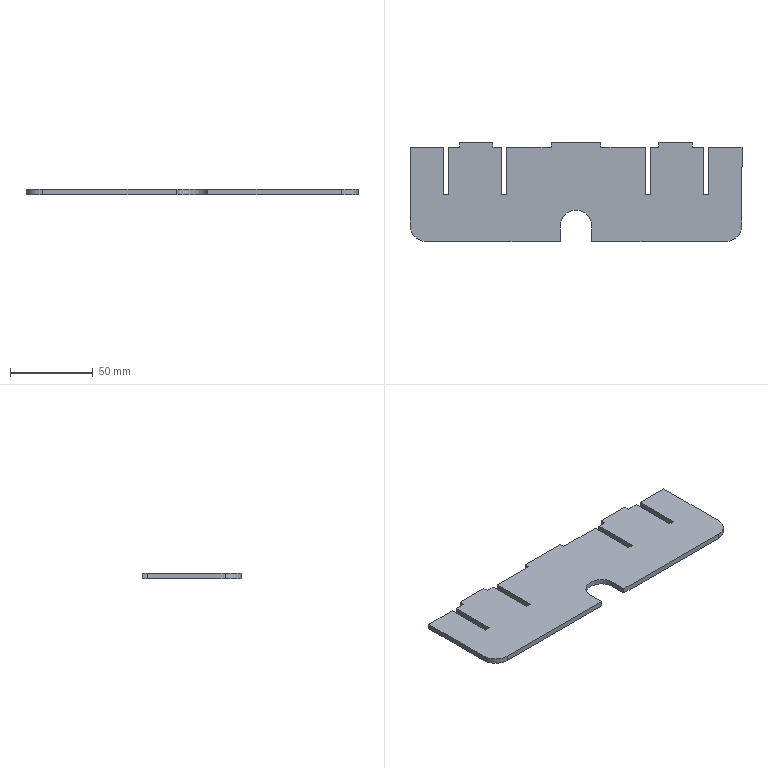Part | SolidWorks | features FlatPattern 1, SMBaseFlange 1, SheetMetal 1 | 1 solid | 40 faces | box 200 x 59.8 x 3.2 mm | volume 34688 mm3 | plane 37 | cylinder 3 | commonest cylinder face diameters 20 x2 19 x1
STEP:
#1=CARTESIAN_POINT('',(166.71,-150.,0.));
#2=VERTEX_POINT('',#1);
#3=CARTESIAN_POINT('',(166.71,-103.2,0.));
#4=VERTEX_POINT('',#3);
#5=CARTESIAN_POINT('',(166.71,-103.2,0.));
#6=DIRECTION('',(0.,1.,0.));
#7=VECTOR('',#6,1000.);
#8=LINE('',#5,#7);
#9=EDGE_CURVE('',#2,#4,#8,.T.);
#10=ORIENTED_EDGE('',*,*,#9,.F.);
#11=CARTESIAN_POINT('',(166.71,-150.,-3.2));
#12=VERTEX_POINT('',#11);
#13=CARTESIAN_POINT('',(166.71,-150.,-3.2));
#14=DIRECTION('',(0.,0.,1.));
#15=VECTOR('',#14,1000.);
#16=LINE('',#13,#15);
#17=EDGE_CURVE('',#12,#2,#16,.T.);
#18=ORIENTED_EDGE('',*,*,#17,.F.);
#19=CARTESIAN_POINT('',(166.71,-103.2,-3.2));
#20=VERTEX_POINT('',#19);
#21=CARTESIAN_POINT('',(166.71,-103.2,-3.2));
#22=DIRECTION('',(0.,1.,0.));
#23=VECTOR('',#22,1000.);
#24=LINE('',#21,#23);
#25=EDGE_CURVE('',#12,#20,#24,.T.);
#26=ORIENTED_EDGE('',*,*,#25,.T.);
#27=CARTESIAN_POINT('',(166.71,-103.2,-3.2));
#28=DIRECTION('',(0.,0.,1.));
#29=VECTOR('',#28,1000.);
#30=LINE('',#27,#29);
#31=EDGE_CURVE('',#20,#4,#30,.T.);
#32=ORIENTED_EDGE('',*,*,#31,.T.);
#33=EDGE_LOOP('',(#10,#18,#26,#32));
#34=FACE_OUTER_BOUND('',#33,.T.);
#35=CARTESIAN_POINT('',(166.71,-103.2,-3.2));
#36=DIRECTION('',(1.,0.,0.));
#37=DIRECTION('',(0.,1.,0.));
#38=AXIS2_PLACEMENT_3D('',#35,#36,#37);
#39=PLANE('',#38);
#40=ADVANCED_FACE('',(#34),#39,.T.);
#41=CARTESIAN_POINT('',(156.71,-160.,0.));
#42=VERTEX_POINT('',#41);
#43=CARTESIAN_POINT('',(156.71,-150.,0.));
#44=DIRECTION('',(0.,0.,1.));
#45=DIRECTION('',(-1.,0.,0.));
#46=AXIS2_PLACEMENT_3D('',#43,#44,#45);
#47=CIRCLE('',#46,10.);
#48=EDGE_CURVE('',#42,#2,#47,.T.);
#49=ORIENTED_EDGE('',*,*,#48,.F.);
#50=CARTESIAN_POINT('',(156.71,-160.,-3.2));
#51=VERTEX_POINT('',#50);
#52=CARTESIAN_POINT('',(156.71,-160.,-3.2));
#53=DIRECTION('',(0.,0.,1.));
#54=VECTOR('',#53,1000.);
#55=LINE('',#52,#54);
#56=EDGE_CURVE('',#51,#42,#55,.T.);
#57=ORIENTED_EDGE('',*,*,#56,.F.);
#58=CARTESIAN_POINT('',(156.71,-150.,-3.2));
#59=DIRECTION('',(0.,0.,1.));
#60=DIRECTION('',(-1.,0.,0.));
#61=AXIS2_PLACEMENT_3D('',#58,#59,#60);
#62=CIRCLE('',#61,10.);
#63=EDGE_CURVE('',#51,#12,#62,.T.);
#64=ORIENTED_EDGE('',*,*,#63,.T.);
#65=ORIENTED_EDGE('',*,*,#17,.T.);
#66=EDGE_LOOP('',(#49,#57,#64,#65));
#67=FACE_OUTER_BOUND('',#66,.T.);
#68=CARTESIAN_POINT('',(156.71,-150.,-3.2));
#69=DIRECTION('',(0.,0.,1.));
#70=DIRECTION('',(1.,0.,0.));
#71=AXIS2_PLACEMENT_3D('',#68,#69,#70);
#72=CYLINDRICAL_SURFACE('',#71,10.);
#73=ADVANCED_FACE('',(#67),#72,.T.);
#74=CARTESIAN_POINT('',(76.21,-160.,0.));
#75=VERTEX_POINT('',#74);
#76=CARTESIAN_POINT('',(156.71,-160.,0.));
#77=DIRECTION('',(1.,0.,0.));
#78=VECTOR('',#77,1000.);
#79=LINE('',#76,#78);
#80=EDGE_CURVE('',#75,#42,#79,.T.);
#81=ORIENTED_EDGE('',*,*,#80,.F.);
#82=CARTESIAN_POINT('',(76.21,-160.,-3.2));
#83=VERTEX_POINT('',#82);
#84=CARTESIAN_POINT('',(76.21,-160.,-3.2));
#85=DIRECTION('',(0.,0.,1.));
#86=VECTOR('',#85,1000.);
#87=LINE('',#84,#86);
#88=EDGE_CURVE('',#83,#75,#87,.T.);
#89=ORIENTED_EDGE('',*,*,#88,.F.);
#90=CARTESIAN_POINT('',(156.71,-160.,-3.2));
#91=DIRECTION('',(1.,0.,0.));
#92=VECTOR('',#91,1000.);
#93=LINE('',#90,#92);
#94=EDGE_CURVE('',#83,#51,#93,.T.);
#95=ORIENTED_EDGE('',*,*,#94,.T.);
#96=ORIENTED_EDGE('',*,*,#56,.T.);
#97=EDGE_LOOP('',(#81,#89,#95,#96));
#98=FACE_OUTER_BOUND('',#97,.T.);
#99=CARTESIAN_POINT('',(156.71,-160.,-3.2));
#100=DIRECTION('',(0.,-1.,0.));
#101=DIRECTION('',(0.,0.,-1.));
#102=AXIS2_PLACEMENT_3D('',#99,#100,#101);
#103=PLANE('',#102);
#104=ADVANCED_FACE('',(#98),#103,.T.);
#105=CARTESIAN_POINT('',(76.21,-150.5,0.));
#106=VERTEX_POINT('',#105);
#107=CARTESIAN_POINT('',(76.21,-160.,0.));
#108=DIRECTION('',(0.,-1.,0.));
#109=VECTOR('',#108,1000.);
#110=LINE('',#107,#109);
#111=EDGE_CURVE('',#106,#75,#110,.T.);
#112=ORIENTED_EDGE('',*,*,#111,.F.);
#113=CARTESIAN_POINT('',(76.21,-150.5,-3.2));
#114=VERTEX_POINT('',#113);
#115=CARTESIAN_POINT('',(76.21,-150.5,-3.2));
#116=DIRECTION('',(0.,0.,1.));
#117=VECTOR('',#116,1000.);
#118=LINE('',#115,#117);
#119=EDGE_CURVE('',#114,#106,#118,.T.);
#120=ORIENTED_EDGE('',*,*,#119,.F.);
#121=CARTESIAN_POINT('',(76.21,-160.,-3.2));
#122=DIRECTION('',(0.,-1.,0.));
#123=VECTOR('',#122,1000.);
#124=LINE('',#121,#123);
#125=EDGE_CURVE('',#114,#83,#124,.T.);
#126=ORIENTED_EDGE('',*,*,#125,.T.);
#127=ORIENTED_EDGE('',*,*,#88,.T.);
#128=EDGE_LOOP('',(#112,#120,#126,#127));
#129=FACE_OUTER_BOUND('',#128,.T.);
#130=CARTESIAN_POINT('',(76.21,-160.,-3.2));
#131=DIRECTION('',(-1.,0.,0.));
#132=DIRECTION('',(0.,-1.,0.));
#133=AXIS2_PLACEMENT_3D('',#130,#131,#132);
#134=PLANE('',#133);
#135=ADVANCED_FACE('',(#129),#134,.T.);
#136=CARTESIAN_POINT('',(57.21,-150.5,0.));
#137=VERTEX_POINT('',#136);
#138=CARTESIAN_POINT('',(66.71,-150.5,0.));
#139=DIRECTION('',(0.,0.,-1.));
#140=DIRECTION('',(1.,0.,0.));
#141=AXIS2_PLACEMENT_3D('',#138,#139,#140);
#142=CIRCLE('',#141,9.5);
#143=EDGE_CURVE('',#137,#106,#142,.T.);
#144=ORIENTED_EDGE('',*,*,#143,.F.);
#145=CARTESIAN_POINT('',(57.21,-150.5,-3.2));
#146=VERTEX_POINT('',#145);
#147=CARTESIAN_POINT('',(57.21,-150.5,-3.2));
#148=DIRECTION('',(0.,0.,1.));
#149=VECTOR('',#148,1000.);
#150=LINE('',#147,#149);
#151=EDGE_CURVE('',#146,#137,#150,.T.);
#152=ORIENTED_EDGE('',*,*,#151,.F.);
#153=CARTESIAN_POINT('',(66.71,-150.5,-3.2));
#154=DIRECTION('',(0.,0.,-1.));
#155=DIRECTION('',(1.,0.,0.));
#156=AXIS2_PLACEMENT_3D('',#153,#154,#155);
#157=CIRCLE('',#156,9.5);
#158=EDGE_CURVE('',#146,#114,#157,.T.);
#159=ORIENTED_EDGE('',*,*,#158,.T.);
#160=ORIENTED_EDGE('',*,*,#119,.T.);
#161=EDGE_LOOP('',(#144,#152,#159,#160));
#162=FACE_OUTER_BOUND('',#161,.T.);
#163=CARTESIAN_POINT('',(66.71,-150.5,-3.2));
#164=DIRECTION('',(0.,0.,1.));
#165=DIRECTION('',(1.,0.,0.));
#166=AXIS2_PLACEMENT_3D('',#163,#164,#165);
#167=CYLINDRICAL_SURFACE('',#166,9.5);
#168=ADVANCED_FACE('',(#162),#167,.F.);
#169=CARTESIAN_POINT('',(57.21,-160.,0.));
#170=VERTEX_POINT('',#169);
#171=CARTESIAN_POINT('',(57.21,-150.5,0.));
#172=DIRECTION('',(0.,1.,0.));
#173=VECTOR('',#172,1000.);
#174=LINE('',#171,#173);
#175=EDGE_CURVE('',#170,#137,#174,.T.);
#176=ORIENTED_EDGE('',*,*,#175,.F.);
#177=CARTESIAN_POINT('',(57.21,-160.,-3.2));
#178=VERTEX_POINT('',#177);
#179=CARTESIAN_POINT('',(57.21,-160.,-3.2));
#180=DIRECTION('',(0.,0.,1.));
#181=VECTOR('',#180,1000.);
#182=LINE('',#179,#181);
#183=EDGE_CURVE('',#178,#170,#182,.T.);
#184=ORIENTED_EDGE('',*,*,#183,.F.);
#185=CARTESIAN_POINT('',(57.21,-150.5,-3.2));
#186=DIRECTION('',(0.,1.,0.));
#187=VECTOR('',#186,1000.);
#188=LINE('',#185,#187);
#189=EDGE_CURVE('',#178,#146,#188,.T.);
#190=ORIENTED_EDGE('',*,*,#189,.T.);
#191=ORIENTED_EDGE('',*,*,#151,.T.);
#192=EDGE_LOOP('',(#176,#184,#190,#191));
#193=FACE_OUTER_BOUND('',#192,.T.);
#194=CARTESIAN_POINT('',(57.21,-150.5,-3.2));
#195=DIRECTION('',(1.,0.,0.));
#196=DIRECTION('',(0.,1.,0.));
#197=AXIS2_PLACEMENT_3D('',#194,#195,#196);
#198=PLANE('',#197);
#199=ADVANCED_FACE('',(#193),#198,.T.);
#200=CARTESIAN_POINT('',(-23.29,-160.,0.));
#201=VERTEX_POINT('',#200);
#202=CARTESIAN_POINT('',(57.21,-160.,0.));
#203=DIRECTION('',(1.,0.,0.));
#204=VECTOR('',#203,1000.);
#205=LINE('',#202,#204);
#206=EDGE_CURVE('',#201,#170,#205,.T.);
#207=ORIENTED_EDGE('',*,*,#206,.F.);
#208=CARTESIAN_POINT('',(-23.29,-160.,-3.2));
#209=VERTEX_POINT('',#208);
#210=CARTESIAN_POINT('',(-23.29,-160.,-3.2));
#211=DIRECTION('',(0.,0.,1.));
#212=VECTOR('',#211,1000.);
#213=LINE('',#210,#212);
#214=EDGE_CURVE('',#209,#201,#213,.T.);
#215=ORIENTED_EDGE('',*,*,#214,.F.);
#216=CARTESIAN_POINT('',(57.21,-160.,-3.2));
#217=DIRECTION('',(1.,0.,0.));
#218=VECTOR('',#217,1000.);
#219=LINE('',#216,#218);
#220=EDGE_CURVE('',#209,#178,#219,.T.);
#221=ORIENTED_EDGE('',*,*,#220,.T.);
#222=ORIENTED_EDGE('',*,*,#183,.T.);
#223=EDGE_LOOP('',(#207,#215,#221,#222));
#224=FACE_OUTER_BOUND('',#223,.T.);
#225=CARTESIAN_POINT('',(57.21,-160.,-3.2));
#226=DIRECTION('',(0.,-1.,0.));
#227=DIRECTION('',(0.,0.,-1.));
#228=AXIS2_PLACEMENT_3D('',#225,#226,#227);
#229=PLANE('',#228);
#230=ADVANCED_FACE('',(#224),#229,.T.);
#231=CARTESIAN_POINT('',(-33.29,-150.,0.));
#232=VERTEX_POINT('',#231);
#233=CARTESIAN_POINT('',(-23.29,-150.,0.));
#234=DIRECTION('',(0.,0.,1.));
#235=DIRECTION('',(-1.,0.,0.));
#236=AXIS2_PLACEMENT_3D('',#233,#234,#235);
#237=CIRCLE('',#236,10.);
#238=EDGE_CURVE('',#232,#201,#237,.T.);
#239=ORIENTED_EDGE('',*,*,#238,.F.);
#240=CARTESIAN_POINT('',(-33.29,-150.,-3.2));
#241=VERTEX_POINT('',#240);
#242=CARTESIAN_POINT('',(-33.29,-150.,-3.2));
#243=DIRECTION('',(0.,0.,1.));
#244=VECTOR('',#243,1000.);
#245=LINE('',#242,#244);
#246=EDGE_CURVE('',#241,#232,#245,.T.);
#247=ORIENTED_EDGE('',*,*,#246,.F.);
#248=CARTESIAN_POINT('',(-23.29,-150.,-3.2));
#249=DIRECTION('',(0.,0.,1.));
#250=DIRECTION('',(-1.,0.,0.));
#251=AXIS2_PLACEMENT_3D('',#248,#249,#250);
#252=CIRCLE('',#251,10.);
#253=EDGE_CURVE('',#241,#209,#252,.T.);
#254=ORIENTED_EDGE('',*,*,#253,.T.);
#255=ORIENTED_EDGE('',*,*,#214,.T.);
#256=EDGE_LOOP('',(#239,#247,#254,#255));
#257=FACE_OUTER_BOUND('',#256,.T.);
#258=CARTESIAN_POINT('',(-23.29,-150.,-3.2));
#259=DIRECTION('',(0.,0.,1.));
#260=DIRECTION('',(1.,0.,0.));
#261=AXIS2_PLACEMENT_3D('',#258,#259,#260);
#262=CYLINDRICAL_SURFACE('',#261,10.);
#263=ADVANCED_FACE('',(#257),#262,.T.);
#264=CARTESIAN_POINT('',(-33.29,-103.2,0.));
#265=VERTEX_POINT('',#264);
#266=CARTESIAN_POINT('',(-33.29,-103.2,0.));
#267=DIRECTION('',(0.,-1.,0.));
#268=VECTOR('',#267,1000.);
#269=LINE('',#266,#268);
#270=EDGE_CURVE('',#265,#232,#269,.T.);
#271=ORIENTED_EDGE('',*,*,#270,.F.);
#272=CARTESIAN_POINT('',(-33.29,-103.2,-3.2));
#273=VERTEX_POINT('',#272);
#274=CARTESIAN_POINT('',(-33.29,-103.2,-3.2));
#275=DIRECTION('',(0.,0.,1.));
#276=VECTOR('',#275,1000.);
#277=LINE('',#274,#276);
#278=EDGE_CURVE('',#273,#265,#277,.T.);
#279=ORIENTED_EDGE('',*,*,#278,.F.);
#280=CARTESIAN_POINT('',(-33.29,-103.2,-3.2));
#281=DIRECTION('',(0.,-1.,0.));
#282=VECTOR('',#281,1000.);
#283=LINE('',#280,#282);
#284=EDGE_CURVE('',#273,#241,#283,.T.);
#285=ORIENTED_EDGE('',*,*,#284,.T.);
#286=ORIENTED_EDGE('',*,*,#246,.T.);
#287=EDGE_LOOP('',(#271,#279,#285,#286));
#288=FACE_OUTER_BOUND('',#287,.T.);
#289=CARTESIAN_POINT('',(-33.29,-103.2,-3.2));
#290=DIRECTION('',(-1.,0.,0.));
#291=DIRECTION('',(0.,-1.,0.));
#292=AXIS2_PLACEMENT_3D('',#289,#290,#291);
#293=PLANE('',#292);
#294=ADVANCED_FACE('',(#288),#293,.T.);
#295=CARTESIAN_POINT('',(-13.29,-103.2,0.));
#296=VERTEX_POINT('',#295);
#297=CARTESIAN_POINT('',(-13.29,-103.2,0.));
#298=DIRECTION('',(-1.,0.,0.));
#299=VECTOR('',#298,1000.);
#300=LINE('',#297,#299);
#301=EDGE_CURVE('',#296,#265,#300,.T.);
#302=ORIENTED_EDGE('',*,*,#301,.F.);
#303=CARTESIAN_POINT('',(-13.29,-103.2,-3.2));
#304=VERTEX_POINT('',#303);
#305=CARTESIAN_POINT('',(-13.29,-103.2,-3.2));
#306=DIRECTION('',(0.,0.,1.));
#307=VECTOR('',#306,1000.);
#308=LINE('',#305,#307);
#309=EDGE_CURVE('',#304,#296,#308,.T.);
#310=ORIENTED_EDGE('',*,*,#309,.F.);
#311=CARTESIAN_POINT('',(-13.29,-103.2,-3.2));
#312=DIRECTION('',(-1.,0.,0.));
#313=VECTOR('',#312,1000.);
#314=LINE('',#311,#313);
#315=EDGE_CURVE('',#304,#273,#314,.T.);
#316=ORIENTED_EDGE('',*,*,#315,.T.);
#317=ORIENTED_EDGE('',*,*,#278,.T.);
#318=EDGE_LOOP('',(#302,#310,#316,#317));
#319=FACE_OUTER_BOUND('',#318,.T.);
#320=CARTESIAN_POINT('',(-13.29,-103.2,-3.2));
#321=DIRECTION('',(0.,1.,0.));
#322=DIRECTION('',(-1.,0.,0.));
#323=AXIS2_PLACEMENT_3D('',#320,#321,#322);
#324=PLANE('',#323);
#325=ADVANCED_FACE('',(#319),#324,.T.);
#326=CARTESIAN_POINT('',(-13.29,-131.7,0.));
#327=VERTEX_POINT('',#326);
#328=CARTESIAN_POINT('',(-13.29,-131.7,0.));
#329=DIRECTION('',(0.,1.,0.));
#330=VECTOR('',#329,1000.);
#331=LINE('',#328,#330);
#332=EDGE_CURVE('',#327,#296,#331,.T.);
#333=ORIENTED_EDGE('',*,*,#332,.F.);
#334=CARTESIAN_POINT('',(-13.29,-131.7,-3.2));
#335=VERTEX_POINT('',#334);
#336=CARTESIAN_POINT('',(-13.29,-131.7,-3.2));
#337=DIRECTION('',(0.,0.,1.));
#338=VECTOR('',#337,1000.);
#339=LINE('',#336,#338);
#340=EDGE_CURVE('',#335,#327,#339,.T.);
#341=ORIENTED_EDGE('',*,*,#340,.F.);
#342=CARTESIAN_POINT('',(-13.29,-131.7,-3.2));
#343=DIRECTION('',(0.,1.,0.));
#344=VECTOR('',#343,1000.);
#345=LINE('',#342,#344);
#346=EDGE_CURVE('',#335,#304,#345,.T.);
#347=ORIENTED_EDGE('',*,*,#346,.T.);
#348=ORIENTED_EDGE('',*,*,#309,.T.);
#349=EDGE_LOOP('',(#333,#341,#347,#348));
#350=FACE_OUTER_BOUND('',#349,.T.);
#351=CARTESIAN_POINT('',(-13.29,-131.7,-3.2));
#352=DIRECTION('',(1.,0.,0.));
#353=DIRECTION('',(0.,1.,0.));
#354=AXIS2_PLACEMENT_3D('',#351,#352,#353);
#355=PLANE('',#354);
#356=ADVANCED_FACE('',(#350),#355,.T.);
#357=CARTESIAN_POINT('',(-10.09,-131.7,0.));
#358=VERTEX_POINT('',#357);
#359=CARTESIAN_POINT('',(-10.09,-131.7,0.));
#360=DIRECTION('',(-1.,0.,0.));
#361=VECTOR('',#360,1000.);
#362=LINE('',#359,#361);
#363=EDGE_CURVE('',#358,#327,#362,.T.);
#364=ORIENTED_EDGE('',*,*,#363,.F.);
#365=CARTESIAN_POINT('',(-10.09,-131.7,-3.2));
#366=VERTEX_POINT('',#365);
#367=CARTESIAN_POINT('',(-10.09,-131.7,-3.2));
#368=DIRECTION('',(0.,0.,1.));
#369=VECTOR('',#368,1000.);
#370=LINE('',#367,#369);
#371=EDGE_CURVE('',#366,#358,#370,.T.);
#372=ORIENTED_EDGE('',*,*,#371,.F.);
#373=CARTESIAN_POINT('',(-10.09,-131.7,-3.2));
#374=DIRECTION('',(-1.,0.,0.));
#375=VECTOR('',#374,1000.);
#376=LINE('',#373,#375);
#377=EDGE_CURVE('',#366,#335,#376,.T.);
#378=ORIENTED_EDGE('',*,*,#377,.T.);
#379=ORIENTED_EDGE('',*,*,#340,.T.);
#380=EDGE_LOOP('',(#364,#372,#378,#379));
#381=FACE_OUTER_BOUND('',#380,.T.);
#382=CARTESIAN_POINT('',(-10.09,-131.7,-3.2));
#383=DIRECTION('',(0.,1.,0.));
#384=DIRECTION('',(0.,0.,1.));
#385=AXIS2_PLACEMENT_3D('',#382,#383,#384);
#386=PLANE('',#385);
#387=ADVANCED_FACE('',(#381),#386,.T.);
#388=CARTESIAN_POINT('',(-10.09,-103.2,0.));
#389=VERTEX_POINT('',#388);
#390=CARTESIAN_POINT('',(-10.09,-103.2,0.));
#391=DIRECTION('',(0.,-1.,0.));
#392=VECTOR('',#391,1000.);
#393=LINE('',#390,#392);
#394=EDGE_CURVE('',#389,#358,#393,.T.);
#395=ORIENTED_EDGE('',*,*,#394,.F.);
#396=CARTESIAN_POINT('',(-10.09,-103.2,-3.2));
#397=VERTEX_POINT('',#396);
#398=CARTESIAN_POINT('',(-10.09,-103.2,-3.2));
#399=DIRECTION('',(0.,0.,1.));
#400=VECTOR('',#399,1000.);
#401=LINE('',#398,#400);
#402=EDGE_CURVE('',#397,#389,#401,.T.);
#403=ORIENTED_EDGE('',*,*,#402,.F.);
#404=CARTESIAN_POINT('',(-10.09,-103.2,-3.2));
#405=DIRECTION('',(0.,-1.,0.));
#406=VECTOR('',#405,1000.);
#407=LINE('',#404,#406);
#408=EDGE_CURVE('',#397,#366,#407,.T.);
#409=ORIENTED_EDGE('',*,*,#408,.T.);
#410=ORIENTED_EDGE('',*,*,#371,.T.);
#411=EDGE_LOOP('',(#395,#403,#409,#410));
#412=FACE_OUTER_BOUND('',#411,.T.);
#413=CARTESIAN_POINT('',(-10.09,-103.2,-3.2));
#414=DIRECTION('',(-1.,0.,0.));
#415=DIRECTION('',(0.,-1.,0.));
#416=AXIS2_PLACEMENT_3D('',#413,#414,#415);
#417=PLANE('',#416);
#418=ADVANCED_FACE('',(#412),#417,.T.);
#419=CARTESIAN_POINT('',(-3.29,-103.2,0.));
#420=VERTEX_POINT('',#419);
#421=CARTESIAN_POINT('',(-3.29,-103.2,0.));
#422=DIRECTION('',(-1.,0.,0.));
#423=VECTOR('',#422,1000.);
#424=LINE('',#421,#423);
#425=EDGE_CURVE('',#420,#389,#424,.T.);
#426=ORIENTED_EDGE('',*,*,#425,.F.);
#427=CARTESIAN_POINT('',(-3.29,-103.2,-3.2));
#428=VERTEX_POINT('',#427);
#429=CARTESIAN_POINT('',(-3.29,-103.2,-3.2));
#430=DIRECTION('',(0.,0.,1.));
#431=VECTOR('',#430,1000.);
#432=LINE('',#429,#431);
#433=EDGE_CURVE('',#428,#420,#432,.T.);
#434=ORIENTED_EDGE('',*,*,#433,.F.);
#435=CARTESIAN_POINT('',(-3.29,-103.2,-3.2));
#436=DIRECTION('',(-1.,0.,0.));
#437=VECTOR('',#436,1000.);
#438=LINE('',#435,#437);
#439=EDGE_CURVE('',#428,#397,#438,.T.);
#440=ORIENTED_EDGE('',*,*,#439,.T.);
#441=ORIENTED_EDGE('',*,*,#402,.T.);
#442=EDGE_LOOP('',(#426,#434,#440,#441));
#443=FACE_OUTER_BOUND('',#442,.T.);
#444=CARTESIAN_POINT('',(-3.29,-103.2,-3.2));
#445=DIRECTION('',(0.,1.,0.));
#446=DIRECTION('',(-1.,0.,0.));
#447=AXIS2_PLACEMENT_3D('',#444,#445,#446);
#448=PLANE('',#447);
#449=ADVANCED_FACE('',(#443),#448,.T.);
#450=CARTESIAN_POINT('',(-3.29,-100.2,0.));
#451=VERTEX_POINT('',#450);
#452=CARTESIAN_POINT('',(-3.29,-100.2,0.));
#453=DIRECTION('',(0.,-1.,0.));
#454=VECTOR('',#453,1000.);
#455=LINE('',#452,#454);
#456=EDGE_CURVE('',#451,#420,#455,.T.);
#457=ORIENTED_EDGE('',*,*,#456,.F.);
#458=CARTESIAN_POINT('',(-3.29,-100.2,-3.2));
#459=VERTEX_POINT('',#458);
#460=CARTESIAN_POINT('',(-3.29,-100.2,-3.2));
#461=DIRECTION('',(0.,0.,1.));
#462=VECTOR('',#461,1000.);
#463=LINE('',#460,#462);
#464=EDGE_CURVE('',#459,#451,#463,.T.);
#465=ORIENTED_EDGE('',*,*,#464,.F.);
#466=CARTESIAN_POINT('',(-3.29,-100.2,-3.2));
#467=DIRECTION('',(0.,-1.,0.));
#468=VECTOR('',#467,1000.);
#469=LINE('',#466,#468);
#470=EDGE_CURVE('',#459,#428,#469,.T.);
#471=ORIENTED_EDGE('',*,*,#470,.T.);
#472=ORIENTED_EDGE('',*,*,#433,.T.);
#473=EDGE_LOOP('',(#457,#465,#471,#472));
#474=FACE_OUTER_BOUND('',#473,.T.);
#475=CARTESIAN_POINT('',(-3.29,-100.2,-3.2));
#476=DIRECTION('',(-1.,0.,0.));
#477=DIRECTION('',(0.,-1.,0.));
#478=AXIS2_PLACEMENT_3D('',#475,#476,#477);
#479=PLANE('',#478);
#480=ADVANCED_FACE('',(#474),#479,.T.);
#481=CARTESIAN_POINT('',(16.71,-100.2,0.));
#482=VERTEX_POINT('',#481);
#483=CARTESIAN_POINT('',(16.71,-100.2,0.));
#484=DIRECTION('',(-1.,0.,0.));
#485=VECTOR('',#484,1000.);
#486=LINE('',#483,#485);
#487=EDGE_CURVE('',#482,#451,#486,.T.);
#488=ORIENTED_EDGE('',*,*,#487,.F.);
#489=CARTESIAN_POINT('',(16.71,-100.2,-3.2));
#490=VERTEX_POINT('',#489);
#491=CARTESIAN_POINT('',(16.71,-100.2,-3.2));
#492=DIRECTION('',(0.,0.,1.));
#493=VECTOR('',#492,1000.);
#494=LINE('',#491,#493);
#495=EDGE_CURVE('',#490,#482,#494,.T.);
#496=ORIENTED_EDGE('',*,*,#495,.F.);
#497=CARTESIAN_POINT('',(16.71,-100.2,-3.2));
#498=DIRECTION('',(-1.,0.,0.));
#499=VECTOR('',#498,1000.);
#500=LINE('',#497,#499);
#501=EDGE_CURVE('',#490,#459,#500,.T.);
#502=ORIENTED_EDGE('',*,*,#501,.T.);
#503=ORIENTED_EDGE('',*,*,#464,.T.);
#504=EDGE_LOOP('',(#488,#496,#502,#503));
#505=FACE_OUTER_BOUND('',#504,.T.);
#506=CARTESIAN_POINT('',(16.71,-100.2,-3.2));
#507=DIRECTION('',(0.,1.,0.));
#508=DIRECTION('',(0.,0.,1.));
#509=AXIS2_PLACEMENT_3D('',#506,#507,#508);
#510=PLANE('',#509);
#511=ADVANCED_FACE('',(#505),#510,.T.);
#512=CARTESIAN_POINT('',(16.71,-103.2,0.));
#513=VERTEX_POINT('',#512);
#514=CARTESIAN_POINT('',(16.71,-103.2,0.));
#515=DIRECTION('',(0.,1.,0.));
#516=VECTOR('',#515,1000.);
#517=LINE('',#514,#516);
#518=EDGE_CURVE('',#513,#482,#517,.T.);
#519=ORIENTED_EDGE('',*,*,#518,.F.);
#520=CARTESIAN_POINT('',(16.71,-103.2,-3.2));
#521=VERTEX_POINT('',#520);
#522=CARTESIAN_POINT('',(16.71,-103.2,-3.2));
#523=DIRECTION('',(0.,0.,1.));
#524=VECTOR('',#523,1000.);
#525=LINE('',#522,#524);
#526=EDGE_CURVE('',#521,#513,#525,.T.);
#527=ORIENTED_EDGE('',*,*,#526,.F.);
#528=CARTESIAN_POINT('',(16.71,-103.2,-3.2));
#529=DIRECTION('',(0.,1.,0.));
#530=VECTOR('',#529,1000.);
#531=LINE('',#528,#530);
#532=EDGE_CURVE('',#521,#490,#531,.T.);
#533=ORIENTED_EDGE('',*,*,#532,.T.);
#534=ORIENTED_EDGE('',*,*,#495,.T.);
#535=EDGE_LOOP('',(#519,#527,#533,#534));
#536=FACE_OUTER_BOUND('',#535,.T.);
#537=CARTESIAN_POINT('',(16.71,-103.2,-3.2));
#538=DIRECTION('',(1.,0.,0.));
#539=DIRECTION('',(0.,0.,-1.));
#540=AXIS2_PLACEMENT_3D('',#537,#538,#539);
#541=PLANE('',#540);
#542=ADVANCED_FACE('',(#536),#541,.T.);
#543=CARTESIAN_POINT('',(21.71,-103.2,0.));
#544=VERTEX_POINT('',#543);
#545=CARTESIAN_POINT('',(21.71,-103.2,0.));
#546=DIRECTION('',(-1.,0.,0.));
#547=VECTOR('',#546,1000.);
#548=LINE('',#545,#547);
#549=EDGE_CURVE('',#544,#513,#548,.T.);
#550=ORIENTED_EDGE('',*,*,#549,.F.);
#551=CARTESIAN_POINT('',(21.71,-103.2,-3.2));
#552=VERTEX_POINT('',#551);
#553=CARTESIAN_POINT('',(21.71,-103.2,-3.2));
#554=DIRECTION('',(0.,0.,1.));
#555=VECTOR('',#554,1000.);
#556=LINE('',#553,#555);
#557=EDGE_CURVE('',#552,#544,#556,.T.);
#558=ORIENTED_EDGE('',*,*,#557,.F.);
#559=CARTESIAN_POINT('',(21.71,-103.2,-3.2));
#560=DIRECTION('',(-1.,0.,0.));
#561=VECTOR('',#560,1000.);
#562=LINE('',#559,#561);
#563=EDGE_CURVE('',#552,#521,#562,.T.);
#564=ORIENTED_EDGE('',*,*,#563,.T.);
#565=ORIENTED_EDGE('',*,*,#526,.T.);
#566=EDGE_LOOP('',(#550,#558,#564,#565));
#567=FACE_OUTER_BOUND('',#566,.T.);
#568=CARTESIAN_POINT('',(21.71,-103.2,-3.2));
#569=DIRECTION('',(0.,1.,0.));
#570=DIRECTION('',(-1.,0.,0.));
#571=AXIS2_PLACEMENT_3D('',#568,#569,#570);
#572=PLANE('',#571);
#573=ADVANCED_FACE('',(#567),#572,.T.);
#574=CARTESIAN_POINT('',(21.71,-131.7,0.));
#575=VERTEX_POINT('',#574);
#576=CARTESIAN_POINT('',(21.71,-131.7,0.));
#577=DIRECTION('',(0.,1.,0.));
#578=VECTOR('',#577,1000.);
#579=LINE('',#576,#578);
#580=EDGE_CURVE('',#575,#544,#579,.T.);
#581=ORIENTED_EDGE('',*,*,#580,.F.);
#582=CARTESIAN_POINT('',(21.71,-131.7,-3.2));
#583=VERTEX_POINT('',#582);
#584=CARTESIAN_POINT('',(21.71,-131.7,-3.2));
#585=DIRECTION('',(0.,0.,1.));
#586=VECTOR('',#585,1000.);
#587=LINE('',#584,#586);
#588=EDGE_CURVE('',#583,#575,#587,.T.);
#589=ORIENTED_EDGE('',*,*,#588,.F.);
#590=CARTESIAN_POINT('',(21.71,-131.7,-3.2));
#591=DIRECTION('',(0.,1.,0.));
#592=VECTOR('',#591,1000.);
#593=LINE('',#590,#592);
#594=EDGE_CURVE('',#583,#552,#593,.T.);
#595=ORIENTED_EDGE('',*,*,#594,.T.);
#596=ORIENTED_EDGE('',*,*,#557,.T.);
#597=EDGE_LOOP('',(#581,#589,#595,#596));
#598=FACE_OUTER_BOUND('',#597,.T.);
#599=CARTESIAN_POINT('',(21.71,-131.7,-3.2));
#600=DIRECTION('',(1.,0.,0.));
#601=DIRECTION('',(0.,1.,0.));
#602=AXIS2_PLACEMENT_3D('',#599,#600,#601);
#603=PLANE('',#602);
#604=ADVANCED_FACE('',(#598),#603,.T.);
#605=CARTESIAN_POINT('',(24.91,-131.7,0.));
#606=VERTEX_POINT('',#605);
#607=CARTESIAN_POINT('',(24.91,-131.7,0.));
#608=DIRECTION('',(-1.,0.,0.));
#609=VECTOR('',#608,1000.);
#610=LINE('',#607,#609);
#611=EDGE_CURVE('',#606,#575,#610,.T.);
#612=ORIENTED_EDGE('',*,*,#611,.F.);
#613=CARTESIAN_POINT('',(24.91,-131.7,-3.2));
#614=VERTEX_POINT('',#613);
#615=CARTESIAN_POINT('',(24.91,-131.7,-3.2));
#616=DIRECTION('',(0.,0.,1.));
#617=VECTOR('',#616,1000.);
#618=LINE('',#615,#617);
#619=EDGE_CURVE('',#614,#606,#618,.T.);
#620=ORIENTED_EDGE('',*,*,#619,.F.);
#621=CARTESIAN_POINT('',(24.91,-131.7,-3.2));
#622=DIRECTION('',(-1.,0.,0.));
#623=VECTOR('',#622,1000.);
#624=LINE('',#621,#623);
#625=EDGE_CURVE('',#614,#583,#624,.T.);
#626=ORIENTED_EDGE('',*,*,#625,.T.);
#627=ORIENTED_EDGE('',*,*,#588,.T.);
#628=EDGE_LOOP('',(#612,#620,#626,#627));
#629=FACE_OUTER_BOUND('',#628,.T.);
#630=CARTESIAN_POINT('',(24.91,-131.7,-3.2));
#631=DIRECTION('',(0.,1.,0.));
#632=DIRECTION('',(0.,0.,1.));
#633=AXIS2_PLACEMENT_3D('',#630,#631,#632);
#634=PLANE('',#633);
#635=ADVANCED_FACE('',(#629),#634,.T.);
#636=CARTESIAN_POINT('',(24.91,-103.2,0.));
#637=VERTEX_POINT('',#636);
#638=CARTESIAN_POINT('',(24.91,-103.2,0.));
#639=DIRECTION('',(0.,-1.,0.));
#640=VECTOR('',#639,1000.);
#641=LINE('',#638,#640);
#642=EDGE_CURVE('',#637,#606,#641,.T.);
#643=ORIENTED_EDGE('',*,*,#642,.F.);
#644=CARTESIAN_POINT('',(24.91,-103.2,-3.2));
#645=VERTEX_POINT('',#644);
#646=CARTESIAN_POINT('',(24.91,-103.2,-3.2));
#647=DIRECTION('',(0.,0.,1.));
#648=VECTOR('',#647,1000.);
#649=LINE('',#646,#648);
#650=EDGE_CURVE('',#645,#637,#649,.T.);
#651=ORIENTED_EDGE('',*,*,#650,.F.);
#652=CARTESIAN_POINT('',(24.91,-103.2,-3.2));
#653=DIRECTION('',(0.,-1.,0.));
#654=VECTOR('',#653,1000.);
#655=LINE('',#652,#654);
#656=EDGE_CURVE('',#645,#614,#655,.T.);
#657=ORIENTED_EDGE('',*,*,#656,.T.);
#658=ORIENTED_EDGE('',*,*,#619,.T.);
#659=EDGE_LOOP('',(#643,#651,#657,#658));
#660=FACE_OUTER_BOUND('',#659,.T.);
#661=CARTESIAN_POINT('',(24.91,-103.2,-3.2));
#662=DIRECTION('',(-1.,0.,0.));
#663=DIRECTION('',(0.,-1.,0.));
#664=AXIS2_PLACEMENT_3D('',#661,#662,#663);
#665=PLANE('',#664);
#666=ADVANCED_FACE('',(#660),#665,.T.);
#667=CARTESIAN_POINT('',(51.71,-103.2,0.));
#668=VERTEX_POINT('',#667);
#669=CARTESIAN_POINT('',(51.71,-103.2,0.));
#670=DIRECTION('',(-1.,0.,0.));
#671=VECTOR('',#670,1000.);
#672=LINE('',#669,#671);
#673=EDGE_CURVE('',#668,#637,#672,.T.);
#674=ORIENTED_EDGE('',*,*,#673,.F.);
#675=CARTESIAN_POINT('',(51.71,-103.2,-3.2));
#676=VERTEX_POINT('',#675);
#677=CARTESIAN_POINT('',(51.71,-103.2,-3.2));
#678=DIRECTION('',(0.,0.,1.));
#679=VECTOR('',#678,1000.);
#680=LINE('',#677,#679);
#681=EDGE_CURVE('',#676,#668,#680,.T.);
#682=ORIENTED_EDGE('',*,*,#681,.F.);
#683=CARTESIAN_POINT('',(51.71,-103.2,-3.2));
#684=DIRECTION('',(-1.,0.,0.));
#685=VECTOR('',#684,1000.);
#686=LINE('',#683,#685);
#687=EDGE_CURVE('',#676,#645,#686,.T.);
#688=ORIENTED_EDGE('',*,*,#687,.T.);
#689=ORIENTED_EDGE('',*,*,#650,.T.);
#690=EDGE_LOOP('',(#674,#682,#688,#689));
#691=FACE_OUTER_BOUND('',#690,.T.);
#692=CARTESIAN_POINT('',(51.71,-103.2,-3.2));
#693=DIRECTION('',(0.,1.,0.));
#694=DIRECTION('',(-1.,0.,0.));
#695=AXIS2_PLACEMENT_3D('',#692,#693,#694);
#696=PLANE('',#695);
#697=ADVANCED_FACE('',(#691),#696,.T.);
#698=CARTESIAN_POINT('',(51.71,-100.2,0.));
#699=VERTEX_POINT('',#698);
#700=CARTESIAN_POINT('',(51.71,-100.2,0.));
#701=DIRECTION('',(0.,-1.,0.));
#702=VECTOR('',#701,1000.);
#703=LINE('',#700,#702);
#704=EDGE_CURVE('',#699,#668,#703,.T.);
#705=ORIENTED_EDGE('',*,*,#704,.F.);
#706=CARTESIAN_POINT('',(51.71,-100.2,-3.2));
#707=VERTEX_POINT('',#706);
#708=CARTESIAN_POINT('',(51.71,-100.2,-3.2));
#709=DIRECTION('',(0.,0.,1.));
#710=VECTOR('',#709,1000.);
#711=LINE('',#708,#710);
#712=EDGE_CURVE('',#707,#699,#711,.T.);
#713=ORIENTED_EDGE('',*,*,#712,.F.);
#714=CARTESIAN_POINT('',(51.71,-100.2,-3.2));
#715=DIRECTION('',(0.,-1.,0.));
#716=VECTOR('',#715,1000.);
#717=LINE('',#714,#716);
#718=EDGE_CURVE('',#707,#676,#717,.T.);
#719=ORIENTED_EDGE('',*,*,#718,.T.);
#720=ORIENTED_EDGE('',*,*,#681,.T.);
#721=EDGE_LOOP('',(#705,#713,#719,#720));
#722=FACE_OUTER_BOUND('',#721,.T.);
#723=CARTESIAN_POINT('',(51.71,-100.2,-3.2));
#724=DIRECTION('',(-1.,0.,0.));
#725=DIRECTION('',(0.,0.,1.));
#726=AXIS2_PLACEMENT_3D('',#723,#724,#725);
#727=PLANE('',#726);
#728=ADVANCED_FACE('',(#722),#727,.T.);
#729=CARTESIAN_POINT('',(81.71,-100.2,0.));
#730=VERTEX_POINT('',#729);
#731=CARTESIAN_POINT('',(81.71,-100.2,0.));
#732=DIRECTION('',(-1.,0.,0.));
#733=VECTOR('',#732,1000.);
#734=LINE('',#731,#733);
#735=EDGE_CURVE('',#730,#699,#734,.T.);
#736=ORIENTED_EDGE('',*,*,#735,.F.);
#737=CARTESIAN_POINT('',(81.71,-100.2,-3.2));
#738=VERTEX_POINT('',#737);
#739=CARTESIAN_POINT('',(81.71,-100.2,-3.2));
#740=DIRECTION('',(0.,0.,1.));
#741=VECTOR('',#740,1000.);
#742=LINE('',#739,#741);
#743=EDGE_CURVE('',#738,#730,#742,.T.);
#744=ORIENTED_EDGE('',*,*,#743,.F.);
#745=CARTESIAN_POINT('',(81.71,-100.2,-3.2));
#746=DIRECTION('',(-1.,0.,0.));
#747=VECTOR('',#746,1000.);
#748=LINE('',#745,#747);
#749=EDGE_CURVE('',#738,#707,#748,.T.);
#750=ORIENTED_EDGE('',*,*,#749,.T.);
#751=ORIENTED_EDGE('',*,*,#712,.T.);
#752=EDGE_LOOP('',(#736,#744,#750,#751));
#753=FACE_OUTER_BOUND('',#752,.T.);
#754=CARTESIAN_POINT('',(81.71,-100.2,-3.2));
#755=DIRECTION('',(0.,1.,0.));
#756=DIRECTION('',(0.,0.,1.));
#757=AXIS2_PLACEMENT_3D('',#754,#755,#756);
#758=PLANE('',#757);
#759=ADVANCED_FACE('',(#753),#758,.T.);
#760=CARTESIAN_POINT('',(81.71,-103.2,0.));
#761=VERTEX_POINT('',#760);
#762=CARTESIAN_POINT('',(81.71,-103.2,0.));
#763=DIRECTION('',(0.,1.,0.));
#764=VECTOR('',#763,1000.);
#765=LINE('',#762,#764);
#766=EDGE_CURVE('',#761,#730,#765,.T.);
#767=ORIENTED_EDGE('',*,*,#766,.F.);
#768=CARTESIAN_POINT('',(81.71,-103.2,-3.2));
#769=VERTEX_POINT('',#768);
#770=CARTESIAN_POINT('',(81.71,-103.2,-3.2));
#771=DIRECTION('',(0.,0.,1.));
#772=VECTOR('',#771,1000.);
#773=LINE('',#770,#772);
#774=EDGE_CURVE('',#769,#761,#773,.T.);
#775=ORIENTED_EDGE('',*,*,#774,.F.);
#776=CARTESIAN_POINT('',(81.71,-103.2,-3.2));
#777=DIRECTION('',(0.,1.,0.));
#778=VECTOR('',#777,1000.);
#779=LINE('',#776,#778);
#780=EDGE_CURVE('',#769,#738,#779,.T.);
#781=ORIENTED_EDGE('',*,*,#780,.T.);
#782=ORIENTED_EDGE('',*,*,#743,.T.);
#783=EDGE_LOOP('',(#767,#775,#781,#782));
#784=FACE_OUTER_BOUND('',#783,.T.);
#785=CARTESIAN_POINT('',(81.71,-103.2,-3.2));
#786=DIRECTION('',(1.,0.,0.));
#787=DIRECTION('',(0.,0.,-1.));
#788=AXIS2_PLACEMENT_3D('',#785,#786,#787);
#789=PLANE('',#788);
#790=ADVANCED_FACE('',(#784),#789,.T.);
#791=CARTESIAN_POINT('',(108.51,-103.2,0.));
#792=VERTEX_POINT('',#791);
#793=CARTESIAN_POINT('',(108.51,-103.2,0.));
#794=DIRECTION('',(-1.,0.,0.));
#795=VECTOR('',#794,1000.);
#796=LINE('',#793,#795);
#797=EDGE_CURVE('',#792,#761,#796,.T.);
#798=ORIENTED_EDGE('',*,*,#797,.F.);
#799=CARTESIAN_POINT('',(108.51,-103.2,-3.2));
#800=VERTEX_POINT('',#799);
#801=CARTESIAN_POINT('',(108.51,-103.2,-3.2));
#802=DIRECTION('',(0.,0.,1.));
#803=VECTOR('',#802,1000.);
#804=LINE('',#801,#803);
#805=EDGE_CURVE('',#800,#792,#804,.T.);
#806=ORIENTED_EDGE('',*,*,#805,.F.);
#807=CARTESIAN_POINT('',(108.51,-103.2,-3.2));
#808=DIRECTION('',(-1.,0.,0.));
#809=VECTOR('',#808,1000.);
#810=LINE('',#807,#809);
#811=EDGE_CURVE('',#800,#769,#810,.T.);
#812=ORIENTED_EDGE('',*,*,#811,.T.);
#813=ORIENTED_EDGE('',*,*,#774,.T.);
#814=EDGE_LOOP('',(#798,#806,#812,#813));
#815=FACE_OUTER_BOUND('',#814,.T.);
#816=CARTESIAN_POINT('',(108.51,-103.2,-3.2));
#817=DIRECTION('',(0.,1.,0.));
#818=DIRECTION('',(-1.,0.,0.));
#819=AXIS2_PLACEMENT_3D('',#816,#817,#818);
#820=PLANE('',#819);
#821=ADVANCED_FACE('',(#815),#820,.T.);
#822=CARTESIAN_POINT('',(108.51,-131.7,0.));
#823=VERTEX_POINT('',#822);
#824=CARTESIAN_POINT('',(108.51,-131.7,0.));
#825=DIRECTION('',(0.,1.,0.));
#826=VECTOR('',#825,1000.);
#827=LINE('',#824,#826);
#828=EDGE_CURVE('',#823,#792,#827,.T.);
#829=ORIENTED_EDGE('',*,*,#828,.F.);
#830=CARTESIAN_POINT('',(108.51,-131.7,-3.2));
#831=VERTEX_POINT('',#830);
#832=CARTESIAN_POINT('',(108.51,-131.7,-3.2));
#833=DIRECTION('',(0.,0.,1.));
#834=VECTOR('',#833,1000.);
#835=LINE('',#832,#834);
#836=EDGE_CURVE('',#831,#823,#835,.T.);
#837=ORIENTED_EDGE('',*,*,#836,.F.);
#838=CARTESIAN_POINT('',(108.51,-131.7,-3.2));
#839=DIRECTION('',(0.,1.,0.));
#840=VECTOR('',#839,1000.);
#841=LINE('',#838,#840);
#842=EDGE_CURVE('',#831,#800,#841,.T.);
#843=ORIENTED_EDGE('',*,*,#842,.T.);
#844=ORIENTED_EDGE('',*,*,#805,.T.);
#845=EDGE_LOOP('',(#829,#837,#843,#844));
#846=FACE_OUTER_BOUND('',#845,.T.);
#847=CARTESIAN_POINT('',(108.51,-131.7,-3.2));
#848=DIRECTION('',(1.,0.,0.));
#849=DIRECTION('',(0.,1.,0.));
#850=AXIS2_PLACEMENT_3D('',#847,#848,#849);
#851=PLANE('',#850);
#852=ADVANCED_FACE('',(#846),#851,.T.);
#853=CARTESIAN_POINT('',(111.71,-131.7,0.));
#854=VERTEX_POINT('',#853);
#855=CARTESIAN_POINT('',(111.71,-131.7,0.));
#856=DIRECTION('',(-1.,0.,0.));
#857=VECTOR('',#856,1000.);
#858=LINE('',#855,#857);
#859=EDGE_CURVE('',#854,#823,#858,.T.);
#860=ORIENTED_EDGE('',*,*,#859,.F.);
#861=CARTESIAN_POINT('',(111.71,-131.7,-3.2));
#862=VERTEX_POINT('',#861);
#863=CARTESIAN_POINT('',(111.71,-131.7,-3.2));
#864=DIRECTION('',(0.,0.,1.));
#865=VECTOR('',#864,1000.);
#866=LINE('',#863,#865);
#867=EDGE_CURVE('',#862,#854,#866,.T.);
#868=ORIENTED_EDGE('',*,*,#867,.F.);
#869=CARTESIAN_POINT('',(111.71,-131.7,-3.2));
#870=DIRECTION('',(-1.,0.,0.));
#871=VECTOR('',#870,1000.);
#872=LINE('',#869,#871);
#873=EDGE_CURVE('',#862,#831,#872,.T.);
#874=ORIENTED_EDGE('',*,*,#873,.T.);
#875=ORIENTED_EDGE('',*,*,#836,.T.);
#876=EDGE_LOOP('',(#860,#868,#874,#875));
#877=FACE_OUTER_BOUND('',#876,.T.);
#878=CARTESIAN_POINT('',(111.71,-131.7,-3.2));
#879=DIRECTION('',(0.,1.,0.));
#880=DIRECTION('',(0.,0.,1.));
#881=AXIS2_PLACEMENT_3D('',#878,#879,#880);
#882=PLANE('',#881);
#883=ADVANCED_FACE('',(#877),#882,.T.);
#884=CARTESIAN_POINT('',(111.71,-103.2,0.));
#885=VERTEX_POINT('',#884);
#886=CARTESIAN_POINT('',(111.71,-103.2,0.));
#887=DIRECTION('',(0.,-1.,0.));
#888=VECTOR('',#887,1000.);
#889=LINE('',#886,#888);
#890=EDGE_CURVE('',#885,#854,#889,.T.);
#891=ORIENTED_EDGE('',*,*,#890,.F.);
#892=CARTESIAN_POINT('',(111.71,-103.2,-3.2));
#893=VERTEX_POINT('',#892);
#894=CARTESIAN_POINT('',(111.71,-103.2,-3.2));
#895=DIRECTION('',(0.,0.,1.));
#896=VECTOR('',#895,1000.);
#897=LINE('',#894,#896);
#898=EDGE_CURVE('',#893,#885,#897,.T.);
#899=ORIENTED_EDGE('',*,*,#898,.F.);
#900=CARTESIAN_POINT('',(111.71,-103.2,-3.2));
#901=DIRECTION('',(0.,-1.,0.));
#902=VECTOR('',#901,1000.);
#903=LINE('',#900,#902);
#904=EDGE_CURVE('',#893,#862,#903,.T.);
#905=ORIENTED_EDGE('',*,*,#904,.T.);
#906=ORIENTED_EDGE('',*,*,#867,.T.);
#907=EDGE_LOOP('',(#891,#899,#905,#906));
#908=FACE_OUTER_BOUND('',#907,.T.);
#909=CARTESIAN_POINT('',(111.71,-103.2,-3.2));
#910=DIRECTION('',(-1.,0.,0.));
#911=DIRECTION('',(0.,-1.,0.));
#912=AXIS2_PLACEMENT_3D('',#909,#910,#911);
#913=PLANE('',#912);
#914=ADVANCED_FACE('',(#908),#913,.T.);
#915=CARTESIAN_POINT('',(116.71,-103.2,0.));
#916=VERTEX_POINT('',#915);
#917=CARTESIAN_POINT('',(116.71,-103.2,0.));
#918=DIRECTION('',(-1.,0.,0.));
#919=VECTOR('',#918,1000.);
#920=LINE('',#917,#919);
#921=EDGE_CURVE('',#916,#885,#920,.T.);
#922=ORIENTED_EDGE('',*,*,#921,.F.);
#923=CARTESIAN_POINT('',(116.71,-103.2,-3.2));
#924=VERTEX_POINT('',#923);
#925=CARTESIAN_POINT('',(116.71,-103.2,-3.2));
#926=DIRECTION('',(0.,0.,1.));
#927=VECTOR('',#926,1000.);
#928=LINE('',#925,#927);
#929=EDGE_CURVE('',#924,#916,#928,.T.);
#930=ORIENTED_EDGE('',*,*,#929,.F.);
#931=CARTESIAN_POINT('',(116.71,-103.2,-3.2));
#932=DIRECTION('',(-1.,0.,0.));
#933=VECTOR('',#932,1000.);
#934=LINE('',#931,#933);
#935=EDGE_CURVE('',#924,#893,#934,.T.);
#936=ORIENTED_EDGE('',*,*,#935,.T.);
#937=ORIENTED_EDGE('',*,*,#898,.T.);
#938=EDGE_LOOP('',(#922,#930,#936,#937));
#939=FACE_OUTER_BOUND('',#938,.T.);
#940=CARTESIAN_POINT('',(116.71,-103.2,-3.2));
#941=DIRECTION('',(0.,1.,0.));
#942=DIRECTION('',(-1.,0.,0.));
#943=AXIS2_PLACEMENT_3D('',#940,#941,#942);
#944=PLANE('',#943);
#945=ADVANCED_FACE('',(#939),#944,.T.);
#946=CARTESIAN_POINT('',(116.71,-100.2,0.));
#947=VERTEX_POINT('',#946);
#948=CARTESIAN_POINT('',(116.71,-100.2,0.));
#949=DIRECTION('',(0.,-1.,0.));
#950=VECTOR('',#949,1000.);
#951=LINE('',#948,#950);
#952=EDGE_CURVE('',#947,#916,#951,.T.);
#953=ORIENTED_EDGE('',*,*,#952,.F.);
#954=CARTESIAN_POINT('',(116.71,-100.2,-3.2));
#955=VERTEX_POINT('',#954);
#956=CARTESIAN_POINT('',(116.71,-100.2,-3.2));
#957=DIRECTION('',(0.,0.,1.));
#958=VECTOR('',#957,1000.);
#959=LINE('',#956,#958);
#960=EDGE_CURVE('',#955,#947,#959,.T.);
#961=ORIENTED_EDGE('',*,*,#960,.F.);
#962=CARTESIAN_POINT('',(116.71,-100.2,-3.2));
#963=DIRECTION('',(0.,-1.,0.));
#964=VECTOR('',#963,1000.);
#965=LINE('',#962,#964);
#966=EDGE_CURVE('',#955,#924,#965,.T.);
#967=ORIENTED_EDGE('',*,*,#966,.T.);
#968=ORIENTED_EDGE('',*,*,#929,.T.);
#969=EDGE_LOOP('',(#953,#961,#967,#968));
#970=FACE_OUTER_BOUND('',#969,.T.);
#971=CARTESIAN_POINT('',(116.71,-100.2,-3.2));
#972=DIRECTION('',(-1.,0.,0.));
#973=DIRECTION('',(0.,0.,1.));
#974=AXIS2_PLACEMENT_3D('',#971,#972,#973);
#975=PLANE('',#974);
#976=ADVANCED_FACE('',(#970),#975,.T.);
#977=CARTESIAN_POINT('',(136.71,-100.2,0.));
#978=VERTEX_POINT('',#977);
#979=CARTESIAN_POINT('',(136.71,-100.2,0.));
#980=DIRECTION('',(-1.,0.,0.));
#981=VECTOR('',#980,1000.);
#982=LINE('',#979,#981);
#983=EDGE_CURVE('',#978,#947,#982,.T.);
#984=ORIENTED_EDGE('',*,*,#983,.F.);
#985=CARTESIAN_POINT('',(136.71,-100.2,-3.2));
#986=VERTEX_POINT('',#985);
#987=CARTESIAN_POINT('',(136.71,-100.2,-3.2));
#988=DIRECTION('',(0.,0.,1.));
#989=VECTOR('',#988,1000.);
#990=LINE('',#987,#989);
#991=EDGE_CURVE('',#986,#978,#990,.T.);
#992=ORIENTED_EDGE('',*,*,#991,.F.);
#993=CARTESIAN_POINT('',(136.71,-100.2,-3.2));
#994=DIRECTION('',(-1.,0.,0.));
#995=VECTOR('',#994,1000.);
#996=LINE('',#993,#995);
#997=EDGE_CURVE('',#986,#955,#996,.T.);
#998=ORIENTED_EDGE('',*,*,#997,.T.);
#999=ORIENTED_EDGE('',*,*,#960,.T.);
#1000=EDGE_LOOP('',(#984,#992,#998,#999));
#1001=FACE_OUTER_BOUND('',#1000,.T.);
#1002=CARTESIAN_POINT('',(136.71,-100.2,-3.2));
#1003=DIRECTION('',(0.,1.,0.));
#1004=DIRECTION('',(0.,0.,1.));
#1005=AXIS2_PLACEMENT_3D('',#1002,#1003,#1004);
#1006=PLANE('',#1005);
#1007=ADVANCED_FACE('',(#1001),#1006,.T.);
#1008=CARTESIAN_POINT('',(136.71,-103.2,0.));
#1009=VERTEX_POINT('',#1008);
#1010=CARTESIAN_POINT('',(136.71,-103.2,0.));
#1011=DIRECTION('',(0.,1.,0.));
#1012=VECTOR('',#1011,1000.);
#1013=LINE('',#1010,#1012);
#1014=EDGE_CURVE('',#1009,#978,#1013,.T.);
#1015=ORIENTED_EDGE('',*,*,#1014,.F.);
#1016=CARTESIAN_POINT('',(136.71,-103.2,-3.2));
#1017=VERTEX_POINT('',#1016);
#1018=CARTESIAN_POINT('',(136.71,-103.2,-3.2));
#1019=DIRECTION('',(0.,0.,1.));
#1020=VECTOR('',#1019,1000.);
#1021=LINE('',#1018,#1020);
#1022=EDGE_CURVE('',#1017,#1009,#1021,.T.);
#1023=ORIENTED_EDGE('',*,*,#1022,.F.);
#1024=CARTESIAN_POINT('',(136.71,-103.2,-3.2));
#1025=DIRECTION('',(0.,1.,0.));
#1026=VECTOR('',#1025,1000.);
#1027=LINE('',#1024,#1026);
#1028=EDGE_CURVE('',#1017,#986,#1027,.T.);
#1029=ORIENTED_EDGE('',*,*,#1028,.T.);
#1030=ORIENTED_EDGE('',*,*,#991,.T.);
#1031=EDGE_LOOP('',(#1015,#1023,#1029,#1030));
#1032=FACE_OUTER_BOUND('',#1031,.T.);
#1033=CARTESIAN_POINT('',(136.71,-103.2,-3.2));
#1034=DIRECTION('',(1.,0.,0.));
#1035=DIRECTION('',(0.,0.,-1.));
#1036=AXIS2_PLACEMENT_3D('',#1033,#1034,#1035);
#1037=PLANE('',#1036);
#1038=ADVANCED_FACE('',(#1032),#1037,.T.);
#1039=CARTESIAN_POINT('',(143.51,-103.2,0.));
#1040=VERTEX_POINT('',#1039);
#1041=CARTESIAN_POINT('',(143.51,-103.2,0.));
#1042=DIRECTION('',(-1.,0.,0.));
#1043=VECTOR('',#1042,1000.);
#1044=LINE('',#1041,#1043);
#1045=EDGE_CURVE('',#1040,#1009,#1044,.T.);
#1046=ORIENTED_EDGE('',*,*,#1045,.F.);
#1047=CARTESIAN_POINT('',(143.51,-103.2,-3.2));
#1048=VERTEX_POINT('',#1047);
#1049=CARTESIAN_POINT('',(143.51,-103.2,-3.2));
#1050=DIRECTION('',(0.,0.,1.));
#1051=VECTOR('',#1050,1000.);
#1052=LINE('',#1049,#1051);
#1053=EDGE_CURVE('',#1048,#1040,#1052,.T.);
#1054=ORIENTED_EDGE('',*,*,#1053,.F.);
#1055=CARTESIAN_POINT('',(143.51,-103.2,-3.2));
#1056=DIRECTION('',(-1.,0.,0.));
#1057=VECTOR('',#1056,1000.);
#1058=LINE('',#1055,#1057);
#1059=EDGE_CURVE('',#1048,#1017,#1058,.T.);
#1060=ORIENTED_EDGE('',*,*,#1059,.T.);
#1061=ORIENTED_EDGE('',*,*,#1022,.T.);
#1062=EDGE_LOOP('',(#1046,#1054,#1060,#1061));
#1063=FACE_OUTER_BOUND('',#1062,.T.);
#1064=CARTESIAN_POINT('',(143.51,-103.2,-3.2));
#1065=DIRECTION('',(0.,1.,0.));
#1066=DIRECTION('',(-1.,0.,0.));
#1067=AXIS2_PLACEMENT_3D('',#1064,#1065,#1066);
#1068=PLANE('',#1067);
#1069=ADVANCED_FACE('',(#1063),#1068,.T.);
#1070=CARTESIAN_POINT('',(143.51,-131.7,0.));
#1071=VERTEX_POINT('',#1070);
#1072=CARTESIAN_POINT('',(143.51,-131.7,0.));
#1073=DIRECTION('',(0.,1.,0.));
#1074=VECTOR('',#1073,1000.);
#1075=LINE('',#1072,#1074);
#1076=EDGE_CURVE('',#1071,#1040,#1075,.T.);
#1077=ORIENTED_EDGE('',*,*,#1076,.F.);
#1078=CARTESIAN_POINT('',(143.51,-131.7,-3.2));
#1079=VERTEX_POINT('',#1078);
#1080=CARTESIAN_POINT('',(143.51,-131.7,-3.2));
#1081=DIRECTION('',(0.,0.,1.));
#1082=VECTOR('',#1081,1000.);
#1083=LINE('',#1080,#1082);
#1084=EDGE_CURVE('',#1079,#1071,#1083,.T.);
#1085=ORIENTED_EDGE('',*,*,#1084,.F.);
#1086=CARTESIAN_POINT('',(143.51,-131.7,-3.2));
#1087=DIRECTION('',(0.,1.,0.));
#1088=VECTOR('',#1087,1000.);
#1089=LINE('',#1086,#1088);
#1090=EDGE_CURVE('',#1079,#1048,#1089,.T.);
#1091=ORIENTED_EDGE('',*,*,#1090,.T.);
#1092=ORIENTED_EDGE('',*,*,#1053,.T.);
#1093=EDGE_LOOP('',(#1077,#1085,#1091,#1092));
#1094=FACE_OUTER_BOUND('',#1093,.T.);
#1095=CARTESIAN_POINT('',(143.51,-131.7,-3.2));
#1096=DIRECTION('',(1.,0.,0.));
#1097=DIRECTION('',(0.,1.,0.));
#1098=AXIS2_PLACEMENT_3D('',#1095,#1096,#1097);
#1099=PLANE('',#1098);
#1100=ADVANCED_FACE('',(#1094),#1099,.T.);
#1101=CARTESIAN_POINT('',(146.71,-131.7,0.));
#1102=VERTEX_POINT('',#1101);
#1103=CARTESIAN_POINT('',(146.71,-131.7,0.));
#1104=DIRECTION('',(-1.,0.,0.));
#1105=VECTOR('',#1104,1000.);
#1106=LINE('',#1103,#1105);
#1107=EDGE_CURVE('',#1102,#1071,#1106,.T.);
#1108=ORIENTED_EDGE('',*,*,#1107,.F.);
#1109=CARTESIAN_POINT('',(146.71,-131.7,-3.2));
#1110=VERTEX_POINT('',#1109);
#1111=CARTESIAN_POINT('',(146.71,-131.7,-3.2));
#1112=DIRECTION('',(0.,0.,1.));
#1113=VECTOR('',#1112,1000.);
#1114=LINE('',#1111,#1113);
#1115=EDGE_CURVE('',#1110,#1102,#1114,.T.);
#1116=ORIENTED_EDGE('',*,*,#1115,.F.);
#1117=CARTESIAN_POINT('',(146.71,-131.7,-3.2));
#1118=DIRECTION('',(-1.,0.,0.));
#1119=VECTOR('',#1118,1000.);
#1120=LINE('',#1117,#1119);
#1121=EDGE_CURVE('',#1110,#1079,#1120,.T.);
#1122=ORIENTED_EDGE('',*,*,#1121,.T.);
#1123=ORIENTED_EDGE('',*,*,#1084,.T.);
#1124=EDGE_LOOP('',(#1108,#1116,#1122,#1123));
#1125=FACE_OUTER_BOUND('',#1124,.T.);
#1126=CARTESIAN_POINT('',(146.71,-131.7,-3.2));
#1127=DIRECTION('',(0.,1.,0.));
#1128=DIRECTION('',(-1.,0.,0.));
#1129=AXIS2_PLACEMENT_3D('',#1126,#1127,#1128);
#1130=PLANE('',#1129);
#1131=ADVANCED_FACE('',(#1125),#1130,.T.);
#1132=CARTESIAN_POINT('',(146.71,-103.2,0.));
#1133=VERTEX_POINT('',#1132);
#1134=CARTESIAN_POINT('',(146.71,-103.2,0.));
#1135=DIRECTION('',(0.,-1.,0.));
#1136=VECTOR('',#1135,1000.);
#1137=LINE('',#1134,#1136);
#1138=EDGE_CURVE('',#1133,#1102,#1137,.T.);
#1139=ORIENTED_EDGE('',*,*,#1138,.F.);
#1140=CARTESIAN_POINT('',(146.71,-103.2,-3.2));
#1141=VERTEX_POINT('',#1140);
#1142=CARTESIAN_POINT('',(146.71,-103.2,-3.2));
#1143=DIRECTION('',(0.,0.,1.));
#1144=VECTOR('',#1143,1000.);
#1145=LINE('',#1142,#1144);
#1146=EDGE_CURVE('',#1141,#1133,#1145,.T.);
#1147=ORIENTED_EDGE('',*,*,#1146,.F.);
#1148=CARTESIAN_POINT('',(146.71,-103.2,-3.2));
#1149=DIRECTION('',(0.,-1.,0.));
#1150=VECTOR('',#1149,1000.);
#1151=LINE('',#1148,#1150);
#1152=EDGE_CURVE('',#1141,#1110,#1151,.T.);
#1153=ORIENTED_EDGE('',*,*,#1152,.T.);
#1154=ORIENTED_EDGE('',*,*,#1115,.T.);
#1155=EDGE_LOOP('',(#1139,#1147,#1153,#1154));
#1156=FACE_OUTER_BOUND('',#1155,.T.);
#1157=CARTESIAN_POINT('',(146.71,-103.2,-3.2));
#1158=DIRECTION('',(-1.,0.,0.));
#1159=DIRECTION('',(0.,-1.,0.));
#1160=AXIS2_PLACEMENT_3D('',#1157,#1158,#1159);
#1161=PLANE('',#1160);
#1162=ADVANCED_FACE('',(#1156),#1161,.T.);
#1163=CARTESIAN_POINT('',(166.71,-103.2,0.));
#1164=DIRECTION('',(-1.,0.,0.));
#1165=VECTOR('',#1164,1000.);
#1166=LINE('',#1163,#1165);
#1167=EDGE_CURVE('',#4,#1133,#1166,.T.);
#1168=ORIENTED_EDGE('',*,*,#1167,.F.);
#1169=ORIENTED_EDGE('',*,*,#31,.F.);
#1170=CARTESIAN_POINT('',(166.71,-103.2,-3.2));
#1171=DIRECTION('',(-1.,0.,0.));
#1172=VECTOR('',#1171,1000.);
#1173=LINE('',#1170,#1172);
#1174=EDGE_CURVE('',#20,#1141,#1173,.T.);
#1175=ORIENTED_EDGE('',*,*,#1174,.T.);
#1176=ORIENTED_EDGE('',*,*,#1146,.T.);
#1177=EDGE_LOOP('',(#1168,#1169,#1175,#1176));
#1178=FACE_OUTER_BOUND('',#1177,.T.);
#1179=CARTESIAN_POINT('',(166.71,-103.2,-3.2));
#1180=DIRECTION('',(0.,1.,0.));
#1181=DIRECTION('',(-1.,0.,0.));
#1182=AXIS2_PLACEMENT_3D('',#1179,#1180,#1181);
#1183=PLANE('',#1182);
#1184=ADVANCED_FACE('',(#1178),#1183,.T.);
#1185=ORIENTED_EDGE('',*,*,#25,.F.);
#1186=ORIENTED_EDGE('',*,*,#63,.F.);
#1187=ORIENTED_EDGE('',*,*,#94,.F.);
#1188=ORIENTED_EDGE('',*,*,#125,.F.);
#1189=ORIENTED_EDGE('',*,*,#158,.F.);
#1190=ORIENTED_EDGE('',*,*,#189,.F.);
#1191=ORIENTED_EDGE('',*,*,#220,.F.);
#1192=ORIENTED_EDGE('',*,*,#253,.F.);
#1193=ORIENTED_EDGE('',*,*,#284,.F.);
#1194=ORIENTED_EDGE('',*,*,#315,.F.);
#1195=ORIENTED_EDGE('',*,*,#346,.F.);
#1196=ORIENTED_EDGE('',*,*,#377,.F.);
#1197=ORIENTED_EDGE('',*,*,#408,.F.);
#1198=ORIENTED_EDGE('',*,*,#439,.F.);
#1199=ORIENTED_EDGE('',*,*,#470,.F.);
#1200=ORIENTED_EDGE('',*,*,#501,.F.);
#1201=ORIENTED_EDGE('',*,*,#532,.F.);
#1202=ORIENTED_EDGE('',*,*,#563,.F.);
#1203=ORIENTED_EDGE('',*,*,#594,.F.);
#1204=ORIENTED_EDGE('',*,*,#625,.F.);
#1205=ORIENTED_EDGE('',*,*,#656,.F.);
#1206=ORIENTED_EDGE('',*,*,#687,.F.);
#1207=ORIENTED_EDGE('',*,*,#718,.F.);
#1208=ORIENTED_EDGE('',*,*,#749,.F.);
#1209=ORIENTED_EDGE('',*,*,#780,.F.);
#1210=ORIENTED_EDGE('',*,*,#811,.F.);
#1211=ORIENTED_EDGE('',*,*,#842,.F.);
#1212=ORIENTED_EDGE('',*,*,#873,.F.);
#1213=ORIENTED_EDGE('',*,*,#904,.F.);
#1214=ORIENTED_EDGE('',*,*,#935,.F.);
#1215=ORIENTED_EDGE('',*,*,#966,.F.);
#1216=ORIENTED_EDGE('',*,*,#997,.F.);
#1217=ORIENTED_EDGE('',*,*,#1028,.F.);
#1218=ORIENTED_EDGE('',*,*,#1059,.F.);
#1219=ORIENTED_EDGE('',*,*,#1090,.F.);
#1220=ORIENTED_EDGE('',*,*,#1121,.F.);
#1221=ORIENTED_EDGE('',*,*,#1152,.F.);
#1222=ORIENTED_EDGE('',*,*,#1174,.F.);
#1223=EDGE_LOOP('',(#1185,#1186,#1187,#1188,#1189,#1190,#1191,#1192,#1193,#1194,#1195,#1196,#1197,#1198,#1199,#1200,#1201,#1202,#1203,#1204,#1205,#1206,#1207,#1208,#1209,#1210,#1211,#1212,#1213,#1214,#1215,#1216,#1217,#1218,#1219,#1220,#1221,#1222));
#1224=FACE_OUTER_BOUND('',#1223,.T.);
#1225=CARTESIAN_POINT('',(156.71,-150.,-3.2));
#1226=DIRECTION('',(0.,0.,-1.));
#1227=DIRECTION('',(-1.,0.,0.));
#1228=AXIS2_PLACEMENT_3D('',#1225,#1226,#1227);
#1229=PLANE('',#1228);
#1230=ADVANCED_FACE('',(#1224),#1229,.T.);
#1231=ORIENTED_EDGE('',*,*,#9,.T.);
#1232=ORIENTED_EDGE('',*,*,#1167,.T.);
#1233=ORIENTED_EDGE('',*,*,#1138,.T.);
#1234=ORIENTED_EDGE('',*,*,#1107,.T.);
#1235=ORIENTED_EDGE('',*,*,#1076,.T.);
#1236=ORIENTED_EDGE('',*,*,#1045,.T.);
#1237=ORIENTED_EDGE('',*,*,#1014,.T.);
#1238=ORIENTED_EDGE('',*,*,#983,.T.);
#1239=ORIENTED_EDGE('',*,*,#952,.T.);
#1240=ORIENTED_EDGE('',*,*,#921,.T.);
#1241=ORIENTED_EDGE('',*,*,#890,.T.);
#1242=ORIENTED_EDGE('',*,*,#859,.T.);
#1243=ORIENTED_EDGE('',*,*,#828,.T.);
#1244=ORIENTED_EDGE('',*,*,#797,.T.);
#1245=ORIENTED_EDGE('',*,*,#766,.T.);
#1246=ORIENTED_EDGE('',*,*,#735,.T.);
#1247=ORIENTED_EDGE('',*,*,#704,.T.);
#1248=ORIENTED_EDGE('',*,*,#673,.T.);
#1249=ORIENTED_EDGE('',*,*,#642,.T.);
#1250=ORIENTED_EDGE('',*,*,#611,.T.);
#1251=ORIENTED_EDGE('',*,*,#580,.T.);
#1252=ORIENTED_EDGE('',*,*,#549,.T.);
#1253=ORIENTED_EDGE('',*,*,#518,.T.);
#1254=ORIENTED_EDGE('',*,*,#487,.T.);
#1255=ORIENTED_EDGE('',*,*,#456,.T.);
#1256=ORIENTED_EDGE('',*,*,#425,.T.);
#1257=ORIENTED_EDGE('',*,*,#394,.T.);
#1258=ORIENTED_EDGE('',*,*,#363,.T.);
#1259=ORIENTED_EDGE('',*,*,#332,.T.);
#1260=ORIENTED_EDGE('',*,*,#301,.T.);
#1261=ORIENTED_EDGE('',*,*,#270,.T.);
#1262=ORIENTED_EDGE('',*,*,#238,.T.);
#1263=ORIENTED_EDGE('',*,*,#206,.T.);
#1264=ORIENTED_EDGE('',*,*,#175,.T.);
#1265=ORIENTED_EDGE('',*,*,#143,.T.);
#1266=ORIENTED_EDGE('',*,*,#111,.T.);
#1267=ORIENTED_EDGE('',*,*,#80,.T.);
#1268=ORIENTED_EDGE('',*,*,#48,.T.);
#1269=EDGE_LOOP('',(#1231,#1232,#1233,#1234,#1235,#1236,#1237,#1238,#1239,#1240,#1241,#1242,#1243,#1244,#1245,#1246,#1247,#1248,#1249,#1250,#1251,#1252,#1253,#1254,#1255,#1256,#1257,#1258,#1259,#1260,#1261,#1262,#1263,#1264,#1265,#1266,#1267,#1268));
#1270=FACE_OUTER_BOUND('',#1269,.T.);
#1271=CARTESIAN_POINT('',(156.71,-150.,0.));
#1272=DIRECTION('',(0.,0.,-1.));
#1273=DIRECTION('',(-1.,0.,0.));
#1274=AXIS2_PLACEMENT_3D('',#1271,#1272,#1273);
#1275=PLANE('',#1274);
#1276=ADVANCED_FACE('',(#1270),#1275,.F.);
#1277=CLOSED_SHELL('',(#40,#73,#104,#135,#168,#199,#230,#263,#294,#325,#356,#387,#418,#449,#480,#511,#542,#573,#604,#635,#666,#697,#728,#759,#790,#821,#852,#883,#914,#945,#976,#1007,#1038,#1069,#1100,#1131,#1162,#1184,#1230,#1276));
#1278=MANIFOLD_SOLID_BREP('',#1277);
#1279=CARTESIAN_POINT('',(0.,0.,0.));
#1280=DIRECTION('',(0.,0.,1.));
#1281=DIRECTION('',(1.,0.,0.));
#1282=AXIS2_PLACEMENT_3D('',#1279,#1280,#1281);
#1283=(LENGTH_UNIT()NAMED_UNIT(*)SI_UNIT(.MILLI.,.METRE.));
#1284=UNCERTAINTY_MEASURE_WITH_UNIT(LENGTH_MEASURE(0.00001),#1283,'','');
#1285=(NAMED_UNIT(*)PLANE_ANGLE_UNIT()SI_UNIT($,.RADIAN.));
#1286=(NAMED_UNIT(*)SI_UNIT($,.STERADIAN.)SOLID_ANGLE_UNIT());
#1287=(GEOMETRIC_REPRESENTATION_CONTEXT(3)GLOBAL_UNCERTAINTY_ASSIGNED_CONTEXT((#1284))GLOBAL_UNIT_ASSIGNED_CONTEXT((#1283,#1285,#1286))REPRESENTATION_CONTEXT('',''));
#1288=ADVANCED_BREP_SHAPE_REPRESENTATION('',(#1278,#1282),#1287);